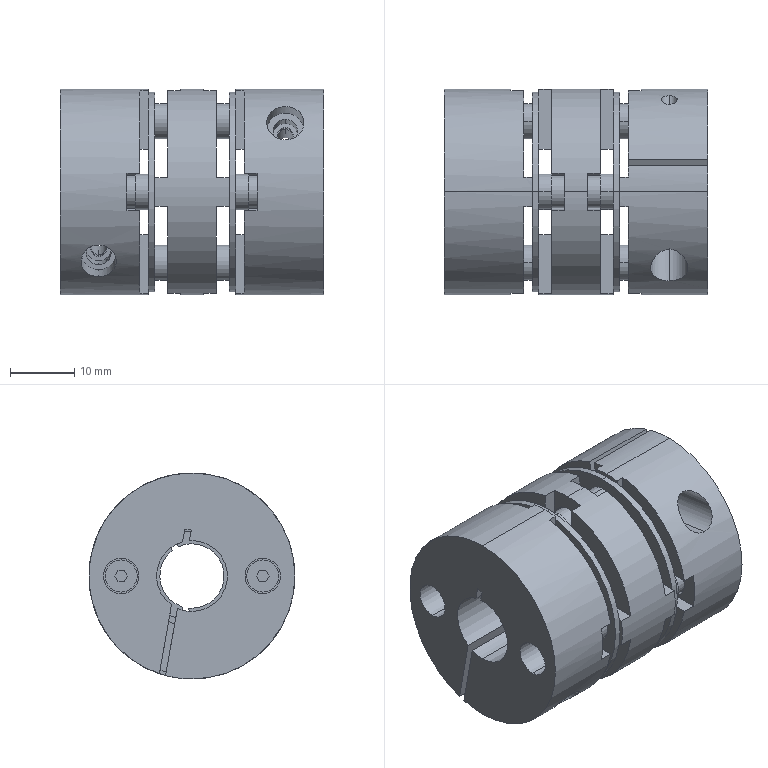Part | STEP file | 001-008-DBA61-D32-d10-e11 | 13 solids | 344 faces | box 41 x 32 x 32 mm | volume 22290 mm3 | plane 164 | cylinder 148 | cone 32 | commonest cylinder face diameters 3 x32 5.5 x30 2.459 x20 5 x16 5.86 x10 14 x10